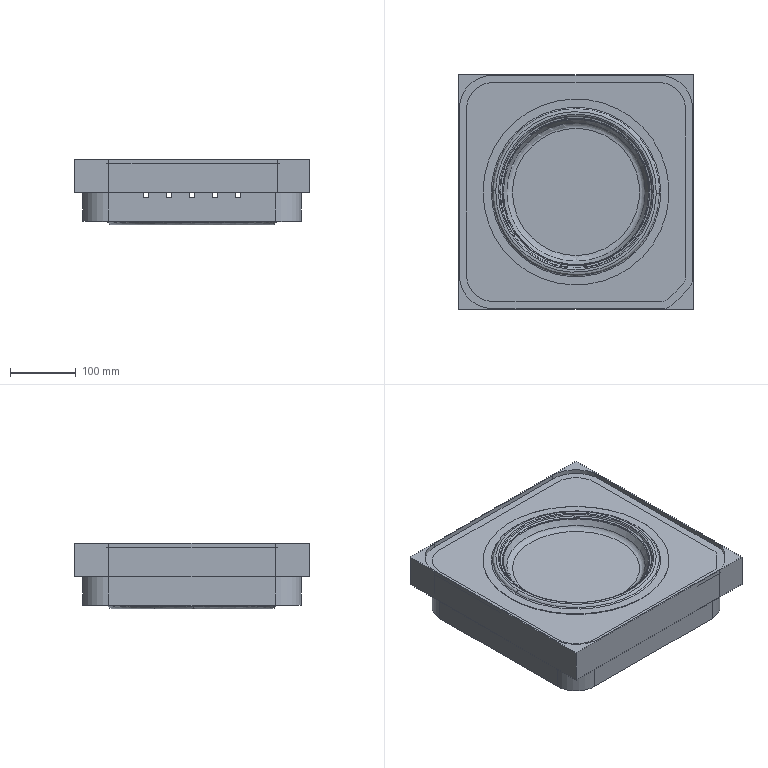NC program | NX | posted with a generic post | part box 356 x 356 x 99.5 mm
Lines 4524 to 5551 of 165566:
(2 , TOOL : D8)
N9046 M6
N9048 G53
N9050 G17 G0 G90 X-104.848 Y1.6 S7000 M3 M8
N9052 G43 Z200.5 H0
N9054 Z48.885
N9056 G94 G1 Z47.885 F4500.
N9058 X-110.089
N9060 G3 X-111.689 Y0. R1.6
N9062 G2 X0. Y111.689 R111.689
N9064 X-111.689 Y0. R-111.689
N9066 G3 X-110.089 Y-1.6 R1.6
N9068 G1 X-104.848
N9070 Z48.885
N9072 G0 Z53.5
N9074 X-104.658 Y1.6
N9076 Z48.556
N9078 G1 Z47.556
N9080 X-109.899
N9082 G3 X-111.499 Y0. R1.6
N9084 G2 X0. Y111.499 R111.499
N9086 X-111.499 Y0. R-111.499
N9088 G3 X-109.899 Y-1.6 R1.6
N9090 G1 X-104.658
N9092 Z48.556
N9094 G0 Z50.885
N9096 X-104.468 Y1.6
N9098 Z48.227
N9100 G1 Z47.227
N9102 X-109.709
N9104 G3 X-111.309 Y0. R1.6
N9106 G2 X0. Y111.309 R111.309
N9108 X-111.309 Y0. R-111.309
N9110 G3 X-109.709 Y-1.6 R1.6
N9112 G1 X-104.468
N9114 Z48.227
N9116 G0 Z50.556
N9118 X-104.278 Y1.6
N9120 Z47.898
N9122 G1 Z46.898
N9124 X-109.519
N9126 G3 X-111.119 Y0. R1.6
N9128 G2 X0. Y111.119 R111.119
N9130 X-111.119 Y0. R-111.119
N9132 G3 X-109.519 Y-1.6 R1.6
N9134 G1 X-104.278
N9136 Z47.898
N9138 G0 Z50.227
N9140 X-104.088 Y1.6
N9142 Z47.569
N9144 G1 Z46.569
N9146 X-109.329
N9148 G3 X-110.929 Y0. R1.6
N9150 G2 X0. Y110.929 R110.929
N9152 X-110.929 Y0. R-110.929
N9154 G3 X-109.329 Y-1.6 R1.6
N9156 G1 X-104.088
N9158 Z47.569
N9160 G0 Z49.898
N9162 X-103.898 Y1.6
N9164 Z47.24
N9166 G1 Z46.24
N9168 X-109.139
N9170 G3 X-110.739 Y0. R1.6
N9172 G2 X0. Y110.739 R110.739
N9174 X-110.739 Y0. R-110.739
N9176 G3 X-109.139 Y-1.6 R1.6
N9178 G1 X-103.898
N9180 Z47.24
N9182 G0 Z49.569
N9184 X-103.709 Y1.6
N9186 Z46.912
N9188 G1 Z45.912
N9190 X-108.945
N9192 G3 X-110.545 Y0. R1.6
N9194 G2 X-0.001 Y110.544 R110.544
N9196 X-110.545 Y0. R-110.544
N9198 G3 X-108.945 Y-1.6 R1.6
N9200 G1 X-103.709
N9202 Z46.912
N9204 G0 Z49.24
N9206 X-102.188 Y1.603
N9208 Z45.678
N9210 G1 Z44.678
N9212 X-107.536
N9214 G3 X-109.136 Y0.003 R1.6
N9216 G2 X1.037 Y109.135 R109.137
N9218 X-55.168 Y-94.163 R-109.134
N9220 X-109.136 Y0.003 R109.137
N9222 G3 X-107.536 Y-1.597 R1.6
N9224 G1 X-102.188
N9226 Z45.678
N9228 G0 Z48.912
N9230 X-72.173 Y-71.373
N9232 Z45.43
N9234 G1 Z44.43
N9236 X-74.264 Y-73.563
N9238 G3 X-74.211 Y-75.825 R1.6
N9240 G1 X-74.196 Y-75.839
N9242 X-74.124 Y-75.908
N9244 G2 X-74.044 Y-78.71 R2.
N9246 G1 X-74.333 Y-78.471
N9248 G3 X-75.025 Y-77.815 R1.538
N9250 G1 X-75.201 Y-77.546
N9252 G2 X-75.894 Y-76.854 R1.441
N9254 X-76.588 Y-76.161 R1.385
N9256 X-77.065 Y-75.802 R1.351
N9258 X-74.299 Y-75.742 R2.
N9260 G1 X-74.211 Y-75.825
N9262 G3 X-71.949 Y-75.772 R1.6
N9264 G1 X-69.853 Y-73.577
N9266 Z45.43
N9268 G0 Z47.678
N9270 X-81.623 Y-60.305
N9272 Z45.43
N9274 G1 Z44.43
N9276 X-83.973 Y-62.37
N9278 G3 X-84.119 Y-64.628 R1.6
N9280 G2 X-83.74 Y-65.106 R6.
N9282 G1 X-83.736 Y-65.111
N9284 G2 X-84.133 Y-67.849 R2.
N9286 X-85.037 Y-66.468 R4.255
N9288 X-86.197 Y-65.083 R2.208
N9290 G1 X-87.205 Y-63.867
N9292 X-87.208 Y-63.839
N9294 G2 X-84.529 Y-64.167 R2.
N9296 G1 X-84.513 Y-64.186
N9298 X-84.147 Y-64.596
N9300 X-84.119 Y-64.628
N9302 G3 X-81.861 Y-64.774 R1.6
N9304 G1 X-79.552 Y-62.744
N9306 Z45.43
N9308 G0 Z47.678
N9310 X-86.432 Y-55.045
N9312 Z45.43
N9314 G1 Z44.43
N9316 X-89.726 Y-57.437
N9318 G3 X-90.08 Y-59.672 R1.6
N9320 X-89.644 Y-60.237 R12.243
N9322 G1 X-89.545 Y-60.542
N9324 X-88.803 Y-61.612
N9326 X-88.76 Y-61.622
N9328 G3 X-87.674 Y-63.006 R6.708
N9330 X-87.609 Y-63.24 R1.008
N9332 X-86.562 Y-63.67 R0.8
N9334 G1 X-80.716 Y-61.232
N9336 Z45.43
N9338 G0 Z47.678
N9340 X-101.427 Y-1.782
N9342 Z45.43
N9344 G1 Z44.43
N9346 X-104.501 Y-1.819
N9348 G3 X-106.081 Y-3.439 R1.6
N9350 G1 X-106.08 Y-3.463
N9352 X-106.079 Y-3.492
N9354 X-106.062 Y-3.809
N9356 G2 X-107.906 Y-5.913 R2.
N9358 X-108.01 Y-4.154 R7.554
N9360 X-107.821 Y-2.077 R3.211
N9362 G1 X-107.825 Y-1.149
N9364 G2 X-106.093 Y-3.068 R2.
N9366 G1 X-106.081 Y-3.439
N9368 G3 X-104.431 Y-4.987 R1.6
N9370 G1 X-101.328 Y-4.888
N9372 Z45.43
N9374 G0 Z47.678
N9376 X-93.646 Y39.774
N9378 Z45.43
N9380 G1 Z44.43
N9382 X-97.306 Y42.148
N9384 G3 X-99.519 Y41.676 R1.6
N9386 G2 X-99.917 Y41.235 R1.875
N9388 G1 X-100.618 Y39.465
N9390 G2 X-101.3 Y37.709 R2.193
N9392 G1 X-101.335 Y37.529
N9394 G3 X-100.07 Y35.653 R1.6
N9396 G1 X-95.614 Y34.786
N9398 Z45.43
N9400 G0 Z47.678
N9402 X-86.878 Y53.863
N9404 Z45.43
N9406 G1 Z44.43
N9408 X-90.305 Y56.034
N9410 G3 X-92.513 Y55.539 R1.6
N9412 G2 X-93.003 Y55.085 R1.302
N9414 X-93.694 Y53.898 R2.033
N9416 X-94.4 Y52.621 R1.816
N9418 G3 X-94.674 Y52.135 R91.572
N9420 X-94.056 Y49.958 R1.6
N9422 G1 X-90.413 Y47.925
N9424 Z45.43
N9426 G0 Z47.678
N9428 X-76.192 Y67.144
N9430 Z45.43
N9432 G1 Z44.43
N9434 X-78.599 Y69.004
N9436 G3 X-80.844 Y68.716 R1.6
N9438 G2 X-80.991 Y68.533 R6.
N9440 X-83.751 Y68.237 R2.
N9442 G1 X-83.453 Y68.545
N9444 G2 X-82.858 Y69.238 R1.082
N9446 X-81.743 Y70.622 R3.617
N9448 X-80.987 Y71.544 R41.003
N9450 X-80.704 Y68.905 R2.
N9452 X-80.844 Y68.716 R6.
N9454 G3 X-80.556 Y66.472 R1.6
N9456 G1 X-78.149 Y64.612
N9458 Z45.43
N9460 G0 Z47.678
N9462 X-75.686 Y68.627
N9464 Z45.43
N9466 G1 Z44.43
N9468 X-78.97 Y71.372
N9470 G3 X-79.077 Y73.632 R1.6
N9472 G1 X-79.087 Y73.641
N9474 G2 X-77.94 Y74.777 R41.003
N9476 X-77.273 Y75.469 R1.379
N9478 X-76.586 Y76.161 R1.377
N9480 X-75.894 Y76.854 R1.384
N9482 X-75.202 Y77.546 R1.411
N9484 X-74.038 Y78.698 R18.413
N9486 X-74.125 Y75.911 R2.
N9488 G1 X-74.204 Y75.835
N9490 X-74.298 Y75.746
N9492 G2 X-75.602 Y75.214 R2.
N9494 X-76.161 Y73.861 R2.
N9496 G1 X-76.29 Y73.726
N9498 G2 X-79.077 Y73.632 R2.
N9500 G3 X-76.817 Y73.74 R1.6
N9502 G1 X-73.96 Y69.454
N9504 Z45.43
N9506 G0 Z47.678
N9508 X72.302 Y71.298
N9510 Z45.43
N9512 G1 Z44.43
N9514 X74.217 Y73.967
N9516 G3 X73.85 Y76.2 R1.6
N9518 G2 X73.63 Y76.383 R2.
N9520 G1 X73.374 Y76.629
N9522 G2 X73.289 Y79.426 R2.
N9524 X74.488 Y78.239 R52.149
N9526 X75.201 Y77.546 R1.572
N9528 X75.894 Y76.854 R1.441
N9530 X76.588 Y76.161 R1.385
N9532 X77.065 Y75.802 R1.351
N9534 X74.298 Y75.743 R2.
N9536 G1 X74.196 Y75.839
N9538 X74.124 Y75.908
N9540 G2 X73.898 Y76.167 R2.
N9542 G1 X73.85 Y76.2
N9544 G3 X71.617 Y75.833 R1.6
N9546 G1 X69.849 Y73.368
N9548 Z45.43
N9550 G0 Z47.678
N9552 X87.184 Y-51.825
N9554 Z45.43
N9556 G1 Z44.43
N9558 X89.811 Y-53.377
N9560 G3 X92.002 Y-52.814 R1.6
N9562 G1 X92.026 Y-52.774
N9564 X92.164 Y-52.544
N9566 G2 X94.85 Y-51.828 R2.
N9568 X93.632 Y-54.005 R113.525
N9570 G3 X93.003 Y-55.085 R1.963
N9572 G1 X92.822 Y-55.39
N9574 X92.599 Y-55.733
N9576 G2 X91.85 Y-53.088 R2.
N9578 X92.002 Y-52.814 R6.
N9580 G3 X91.439 Y-50.622 R1.6
N9582 G1 X88.794 Y-49.059
N9584 Z45.43
N9586 G0 Z47.678
N9588 X75.283 Y-68.769
N9590 Z45.43
N9592 G1 Z44.43
N9594 X78.729 Y-71.73
N9596 G3 X80.986 Y-71.56 R1.6
N9598 X81.77 Y-70.622 R46.024
N9600 X82.858 Y-69.238 R3.911
N9602 X83.453 Y-68.545 R1.082
N9604 G1 X83.737 Y-68.251
N9606 G3 X83.698 Y-65.988 R1.6
N9608 G1 X80.851 Y-63.238
N9610 Z45.43
N9612 G0 Z47.678
N9614 X69.743 Y-73.494
N9616 Z45.43
N9618 G1 Z44.43
N9620 X71.949 Y-75.785
N9622 G3 X74.211 Y-75.828 R1.6
N9624 G1 X74.298 Y-75.746
N9626 G2 X75.602 Y-75.214 R2.
N9628 X76.16 Y-73.862 R2.
N9630 G1 X76.29 Y-73.727
N9632 G2 X79.085 Y-73.639 R2.
N9634 X77.94 Y-74.777 R46.024
N9636 X77.273 Y-75.469 R1.379
N9638 X76.586 Y-76.161 R1.377
N9640 X75.894 Y-76.854 R1.384
N9642 X75.202 Y-77.546 R1.411
N9644 X74.487 Y-78.239 R1.578
N9646 X73.317 Y-79.382 R76.235
N9648 X73.41 Y-76.602 R2.
N9650 G1 X73.602 Y-76.416
N9652 G2 X73.887 Y-76.188 R2.
N9654 X74.125 Y-75.911 R2.
N9656 G1 X74.204 Y-75.835
N9658 X74.211 Y-75.828
N9660 G3 X74.254 Y-73.565 R1.6
N9662 G1 X72.068 Y-71.296
N9664 Z45.43
N9666 G0 Z47.678
N9668 X68.021 Y-71.79
N9670 Z44.242
N9672 G1 Z43.242
N9674 X71.704 Y-75.554
N9676 G3 X73.967 Y-75.578 R1.6
N9678 G2 X-75.578 Y-73.967 R105.75
N9680 X73.967 Y-75.578 R-105.75
N9682 G3 X73.991 Y-73.316 R1.6
N9684 G1 X70.308 Y-69.552
N9686 Z44.242
N9688 G0 Z47.43
N9690 X67.883 Y-71.649
N9692 Z43.9
N9694 G1 Z42.9
N9696 X71.566 Y-75.413
N9698 G3 X73.829 Y-75.437 R1.6
N9700 G2 X-75.437 Y-73.829 R105.553
N9702 X73.829 Y-75.437 R-105.553
N9704 G3 X73.853 Y-73.175 R1.6
N9706 G1 X70.17 Y-69.411
N9708 Z43.9
N9710 G0 Z46.242
N9712 X67.745 Y-71.508
N9714 Z43.559
N9716 G1 Z42.559
N9718 X71.428 Y-75.272
N9720 G3 X73.691 Y-75.296 R1.6
N9722 G2 X-75.296 Y-73.691 R105.356
N9724 X73.691 Y-75.296 R-105.356
N9726 G3 X73.715 Y-73.034 R1.6
N9728 G1 X70.032 Y-69.27
N9730 Z43.559
N9732 G0 Z45.9
N9734 X67.607 Y-71.367
N9736 Z43.217
N9738 G1 Z42.217
N9740 X71.29 Y-75.131
N9742 G3 X73.553 Y-75.155 R1.6
N9744 G2 X-75.155 Y-73.553 R105.159
N9746 X73.553 Y-75.155 R-105.159
N9748 G3 X73.577 Y-72.893 R1.6
N9750 G1 X69.894 Y-69.129
N9752 Z43.217
N9754 G0 Z45.559
N9756 X67.469 Y-71.226
N9758 Z42.875
N9760 G1 Z41.875
N9762 X71.152 Y-74.99
N9764 G3 X73.415 Y-75.014 R1.6
N9766 G2 X-75.014 Y-73.415 R104.962
N9768 X73.415 Y-75.014 R-104.962
N9770 G3 X73.439 Y-72.752 R1.6
N9772 G1 X69.756 Y-68.988
N9774 Z42.875
N9776 G0 Z45.217
N9778 X67.331 Y-71.085
N9780 Z42.534
N9782 G1 Z41.534
N9784 X71.014 Y-74.849
N9786 G3 X73.277 Y-74.873 R1.6
N9788 G2 X-74.873 Y-73.277 R104.764
N9790 X73.277 Y-74.873 R-104.764
N9792 G3 X73.301 Y-72.611 R1.6
N9794 G1 X69.618 Y-68.847
N9796 Z42.534
N9798 G0 Z44.875
N9800 X67.193 Y-70.944
N9802 Z42.192
N9804 G1 Z41.192
N9806 X70.877 Y-74.708
N9808 G3 X73.139 Y-74.733 R1.6
N9810 G2 X-74.733 Y-73.139 R104.567
N9812 X73.139 Y-74.733 R-104.567
N9814 G3 X73.164 Y-72.47 R1.6
N9816 G1 X69.48 Y-68.706
N9818 Z42.192
N9820 G0 Z44.534
N9822 X67.055 Y-70.804
N9824 Z41.851
N9826 G1 Z40.851
N9828 X70.739 Y-74.567
N9830 G3 X73.001 Y-74.592 R1.6
N9832 G2 X-74.592 Y-73.001 R104.37
N9834 X73.001 Y-74.592 R-104.37
N9836 G3 X73.026 Y-72.329 R1.6
N9838 G1 X69.342 Y-68.565
N9840 Z41.851
N9842 G0 Z44.192
N9844 X66.917 Y-70.663
N9846 Z41.509
N9848 G1 Z40.509
N9850 X70.601 Y-74.426
N9852 G3 X72.863 Y-74.451 R1.6
N9854 G2 X-74.451 Y-72.863 R104.173
N9856 X72.863 Y-74.451 R-104.173
N9858 G3 X72.888 Y-72.188 R1.6
N9860 G1 X69.204 Y-68.424
N9862 Z41.509
N9864 G0 Z43.851
N9866 X66.779 Y-70.522
N9868 Z41.168
N9870 G1 Z40.168
N9872 X70.463 Y-74.285
N9874 G3 X72.725 Y-74.31 R1.6
N9876 G2 X-74.31 Y-72.725 R103.976
N9878 X72.725 Y-74.31 R-103.976
N9880 G3 X72.75 Y-72.047 R1.6
N9882 G1 X69.066 Y-68.283
N9884 Z41.168
N9886 G0 Z43.509
N9888 X66.641 Y-70.381
N9890 Z40.826
N9892 G1 Z39.826
N9894 X70.325 Y-74.144
N9896 G3 X72.587 Y-74.169 R1.6
N9898 G2 X-74.169 Y-72.587 R103.778
N9900 X72.587 Y-74.169 R-103.778
N9902 G3 X72.612 Y-71.906 R1.6
N9904 G1 X68.928 Y-68.142
N9906 Z40.826
N9908 G0 Z43.168
N9910 X66.503 Y-70.24
N9912 Z40.484
N9914 G1 Z39.484
N9916 X70.187 Y-74.003
N9918 G3 X72.449 Y-74.028 R1.6
N9920 G2 X-74.028 Y-72.449 R103.581
N9922 X72.449 Y-74.028 R-103.581
N9924 G3 X72.474 Y-71.765 R1.6
N9926 G1 X68.79 Y-68.001
N9928 Z40.484
N9930 G0 Z42.826
N9932 X66.365 Y-70.099
N9934 Z40.143
N9936 G1 Z39.143
N9938 X70.049 Y-73.862
N9940 G3 X72.312 Y-73.887 R1.6
N9942 G2 X-73.887 Y-72.312 R103.384
N9944 X72.312 Y-73.887 R-103.384
N9946 G3 X72.336 Y-71.624 R1.6
N9948 G1 X68.652 Y-67.86
N9950 Z40.143
N9952 G0 Z42.484
N9954 X66.227 Y-69.958
N9956 Z39.801
N9958 G1 Z38.801
N9960 X69.911 Y-73.722
N9962 G3 X72.174 Y-73.746 R1.6
N9964 G2 X-73.746 Y-72.174 R103.187
N9966 X72.174 Y-73.746 R-103.187
N9968 G3 X72.198 Y-71.483 R1.6
N9970 G1 X68.514 Y-67.72
N9972 Z39.801
N9974 G0 Z42.143
N9976 X66.089 Y-69.817
N9978 Z39.46
N9980 G1 Z38.46
N9982 X69.773 Y-73.581
N9984 G3 X72.036 Y-73.605 R1.6
N9986 G2 X-73.605 Y-72.036 R102.989
N9988 X72.036 Y-73.605 R-102.989
N9990 G3 X72.06 Y-71.342 R1.6
N9992 G1 X68.376 Y-67.579
N9994 Z39.46
N9996 G0 Z41.801
N9998 X65.952 Y-69.676
N10000 Z39.118
N10002 G1 Z38.118
N10004 X69.635 Y-73.44
N10006 G3 X71.898 Y-73.464 R1.6
N10008 G2 X-73.464 Y-71.898 R102.792
N10010 X71.898 Y-73.464 R-102.792
N10012 G3 X71.922 Y-71.201 R1.6
N10014 G1 X68.239 Y-67.438
N10016 Z39.118
N10018 G0 Z41.46
N10020 X65.814 Y-69.535
N10022 Z38.776
N10024 G1 Z37.776
N10026 X69.497 Y-73.299
N10028 G3 X71.76 Y-73.323 R1.6
N10030 G2 X-73.323 Y-71.76 R102.595
N10032 X71.76 Y-73.323 R-102.595
N10034 G3 X71.784 Y-71.06 R1.6
N10036 G1 X68.101 Y-67.297
N10038 Z38.776
N10040 G0 Z41.118
N10042 X65.676 Y-69.394
N10044 Z38.435
N10046 G1 Z37.435
N10048 X69.359 Y-73.158
N10050 G3 X71.622 Y-73.182 R1.6
N10052 G2 X-73.182 Y-71.622 R102.398
N10054 X71.622 Y-73.182 R-102.398
N10056 G3 X71.646 Y-70.92 R1.6
N10058 G1 X67.963 Y-67.156
N10060 Z38.435
N10062 G0 Z40.776
N10064 X65.538 Y-69.253
N10066 Z38.093
N10068 G1 Z37.093
N10070 X69.221 Y-73.017
N10072 G3 X71.484 Y-73.041 R1.6
N10074 G2 X-73.041 Y-71.484 R102.201
N10076 X71.484 Y-73.041 R-102.201
N10078 G3 X71.508 Y-70.779 R1.6
N10080 G1 X67.825 Y-67.015
N10082 Z38.093
N10084 G0 Z40.435
N10086 X65.4 Y-69.112
N10088 Z37.752
N10090 G1 Z36.752
N10092 X69.083 Y-72.876
N10094 G3 X71.346 Y-72.9 R1.6
N10096 G2 X-72.9 Y-71.346 R102.003
N10098 X71.346 Y-72.9 R-102.003
N10100 G3 X71.37 Y-70.638 R1.6
N10102 G1 X67.687 Y-66.874
N10104 Z37.752
N10106 G0 Z40.093
N10108 X65.262 Y-68.971
N10110 Z37.41
N10112 G1 Z36.41
N10114 X68.945 Y-72.735
N10116 G3 X71.208 Y-72.759 R1.6
N10118 G2 X-72.759 Y-71.208 R101.806
N10120 X71.208 Y-72.759 R-101.806
N10122 G3 X71.232 Y-70.497 R1.6
N10124 G1 X67.549 Y-66.733
N10126 Z37.41
N10128 G0 Z39.752
N10130 X65.124 Y-68.83
N10132 Z37.069
N10134 G1 Z36.069
N10136 X68.807 Y-72.594
N10138 G3 X71.07 Y-72.618 R1.6
N10140 G2 X-72.618 Y-71.07 R101.609
N10142 X71.07 Y-72.618 R-101.609
N10144 G3 X71.094 Y-70.356 R1.6
N10146 G1 X67.411 Y-66.592
N10148 Z37.069
N10150 G0 Z39.41
N10152 X64.986 Y-68.689
N10154 Z36.727
N10156 G1 Z35.727
N10158 X68.67 Y-72.453
N10160 G3 X70.932 Y-72.477 R1.6
N10162 G2 X-72.477 Y-70.932 R101.412
N10164 X70.932 Y-72.477 R-101.412
N10166 G3 X70.957 Y-70.215 R1.6
N10168 G1 X67.273 Y-66.451
N10170 Z36.727
N10172 G0 Z39.069
N10174 X64.848 Y-68.548
N10176 Z36.385
N10178 G1 Z35.385
N10180 X68.532 Y-72.312
N10182 G3 X70.794 Y-72.336 R1.6
N10184 G2 X-72.336 Y-70.794 R101.215
N10186 X70.794 Y-72.336 R-101.215
N10188 G3 X70.819 Y-70.074 R1.6
N10190 G1 X67.135 Y-66.31
N10192 Z36.385
N10194 G0 Z38.727
N10196 X64.71 Y-68.407
N10198 Z36.044
N10200 G1 Z35.044
N10202 X68.394 Y-72.171
N10204 G3 X70.656 Y-72.196 R1.6
N10206 G2 X-72.196 Y-70.656 R101.017
N10208 X70.656 Y-72.196 R-101.017
N10210 G3 X70.681 Y-69.933 R1.6
N10212 G1 X66.997 Y-66.169
N10214 Z36.044
N10216 G0 Z38.385
N10218 X64.572 Y-68.266
N10220 Z35.702
N10222 G1 Z34.702
N10224 X68.255 Y-72.029
N10226 G3 X70.518 Y-72.054 R1.6
N10228 G2 X-72.054 Y-70.518 R100.819
N10230 X70.518 Y-72.054 R-100.819
N10232 G3 X70.542 Y-69.791 R1.6
N10234 G1 X66.859 Y-66.028
N10236 Z35.702
N10238 G0 Z38.044
N10240 X64.432 Y-68.123
N10242 Z35.361
N10244 G1 Z34.361
N10246 X68.106 Y-71.877
N10248 G3 X70.368 Y-71.901 R1.6
N10250 G2 X-71.901 Y-70.368 R100.606
N10252 X70.368 Y-71.901 R-100.606
N10254 G3 X70.393 Y-69.639 R1.6
N10256 G1 X66.719 Y-65.885
N10258 Z35.361
N10260 G0 Z37.702
N10262 X64.279 Y-67.967
N10264 Z35.019
N10266 G1 Z34.019
N10268 X67.942 Y-71.71
N10270 G3 X70.205 Y-71.734 R1.6
N10272 G2 X-71.734 Y-70.205 R100.372
N10274 X70.205 Y-71.734 R-100.372
N10276 G3 X70.229 Y-69.472 R1.6
N10278 G1 X66.566 Y-65.729
N10280 Z35.019
N10282 G0 Z37.361
N10284 X64.111 Y-67.795
N10286 Z34.677
N10288 G1 Z33.677
N10290 X67.764 Y-71.527
N10292 G3 X70.026 Y-71.552 R1.6
N10294 G2 X-71.552 Y-70.026 R100.116
N10296 X70.026 Y-71.552 R-100.116
N10298 G3 X70.051 Y-69.289 R1.6
N10300 G1 X66.398 Y-65.557
N10302 Z34.677
N10304 G0 Z37.019
N10306 X88.103 Y-1.6
N10308 Z31.262
N10310 G1 Z30.262
N10312 X93.366
N10314 G3 X94.966 Y0. R1.6
N10316 G2 X0. Y-94.966 R94.966
N10318 X94.966 Y0. R-94.966
N10320 G3 X93.366 Y1.6 R1.6
N10322 G1 X88.103
N10324 Z31.262
N10326 G0 Z52.2
N10328 X137.025 Y1.598
N10330 Z47.569
N10332 G1 Z46.569
N10334 X131.798
N10336 G3 X130.198 Y-0.002 R1.6
N10338 G2 X-121.922 Y45.697 R-130.202
N10340 X72.7 Y108.011 R130.201
N10342 X130.198 Y-0.002 R130.202
N10344 G3 X131.798 Y-1.602 R1.6
N10346 G1 X137.026
N10348 Z47.569
N10350 G0 Z49.898
N10352 X137.211 Y1.598
N10354 Z47.24
N10356 G1 Z46.24
N10358 X131.995
N10360 G3 X130.395 Y-0.002 R1.6
N10362 G2 X-0.002 Y-130.395 R130.395
N10364 X130.395 Y-0.002 R-130.395
N10366 G3 X131.995 Y-1.602 R1.6
N10368 G1 X137.21
N10370 Z47.24
N10372 G0 Z49.569
N10374 X137.4 Y1.599
N10376 Z46.912
N10378 G1 Z45.912
N10380 X132.192 Y1.598
N10382 G3 X130.592 Y-0.002 R1.6
N10384 G2 X125.125 Y-37.388 R130.398
N10386 X80.069 Y-103.164 R130.701
N10388 X75.025 Y106.889 R-130.59
N10390 G1 X75.365 Y106.626
N10392 X75.716 Y106.403
N10394 G2 X95.769 Y88.773 R130.593
N10396 X129.34 Y18.002 R130.422
N10398 X130.592 Y-0.002 R130.398
N10400 G3 X132.193 Y-1.602 R1.6
N10402 G1 X137.394 Y-1.601
N10404 Z46.912
N10406 G0 Z49.24
N10408 X152.025 Y1.6
N10410 Z45.678
N10412 G1 Z44.678
N10414 X146.8
N10416 G3 X145.2 Y0. R1.6
N10418 G2 X0. Y-145.2 R145.2
N10420 X145.2 Y0. R-145.2
N10422 G3 X146.8 Y-1.6 R1.6
N10424 G1 X152.025
N10426 Z45.678
N10428 G0 Z47.925
N10430 X152.116 Y1.6
N10432 Z45.43
N10434 G1 Z44.43
N10436 X146.8
N10438 G3 X145.2 Y0. R1.6
N10440 G2 X0. Y-145.2 R145.2
N10442 X145.2 Y0. R-145.2
N10444 G3 X146.8 Y-1.6 R1.6
N10446 G1 X152.116
N10448 Z45.43
N10450 G0 Z47.678
N10452 X152.148 Y1.6
N10454 Z45.178
N10456 G1 Z44.178
N10458 X146.8
N10460 G3 X145.2 Y0. R1.6
N10462 G2 X0. Y-145.2 R145.2
N10464 X145.2 Y0. R-145.2
N10466 G3 X146.8 Y-1.6 R1.6
N10468 G1 X152.148
N10470 Z45.178
N10472 G0 Z47.43
N10474 X152.732 Y1.6
N10476 Z44.925
N10478 G1 Z43.925
N10480 X146.8
N10482 G3 X145.2 Y0. R1.6
N10484 G2 X0. Y-145.2 R145.2
N10486 X145.2 Y0. R-145.2
N10488 G3 X146.8 Y-1.6 R1.6
N10490 G1 X152.732
N10492 Z44.925
N10494 G0 Z47.925
N10496 X165.815 Y-3.493
N10498 Z45.678
N10500 G1 Z44.678
N10502 X171.2
N10504 G3 X172.8 Y-1.893 R1.6
N10506 G1 Y-129.787
N10508 G2 X166.415 Y-145.202 R21.8
N10510 G1 X145.202 Y-166.415
N10512 G2 X129.787 Y-172.8 R21.8
N10514 G1 X-126.
N10516 G2 X-172.8 Y-126. R46.8
N10518 G1 Y126.
N10520 G2 X-126. Y172.8 R46.8
N10522 G1 X126.
N10524 G2 X172.8 Y126. R46.8
N10526 G1 Y-1.893
N10528 G3 X171.2 Y-0.293 R1.6
N10530 G1 X165.815
N10532 Z45.678
N10534 G0 Z47.925
N10536 X165.843 Y-3.493
N10538 Z45.43
N10540 G1 Z44.43
N10542 X171.2
N10544 G3 X172.8 Y-1.893 R1.6
N10546 G1 Y-129.787
N10548 G2 X166.415 Y-145.202 R21.8
N10550 G1 X145.202 Y-166.415
N10552 G2 X129.787 Y-172.8 R21.8
N10554 G1 X-126.
N10556 G2 X-172.8 Y-126. R46.8
N10558 G1 Y126.
N10560 G2 X-126. Y172.8 R46.8
N10562 G1 X126.
N10564 G2 X172.8 Y126. R46.8
N10566 G1 Y-1.893
N10568 G3 X171.2 Y-0.293 R1.6
N10570 G1 X165.843
N10572 Z45.43
N10574 G0 Z47.678
N10576 Y-3.493
N10578 Z45.178
N10580 G1 Z44.178
N10582 X171.2
N10584 G3 X172.8 Y-1.893 R1.6
N10586 G1 Y-129.787
N10588 G2 X166.415 Y-145.202 R21.8
N10590 G1 X145.202 Y-166.415
N10592 G2 X129.787 Y-172.8 R21.8
N10594 G1 X-126.
N10596 G2 X-172.8 Y-126. R46.8
N10598 G1 Y126.
N10600 G2 X-126. Y172.8 R46.8
N10602 G1 X126.
N10604 G2 X172.8 Y126. R46.8
N10606 G1 Y-1.893
N10608 G3 X171.2 Y-0.293 R1.6
N10610 G1 X165.843
N10612 Z45.178
N10614 G0 Z47.43
N10616 X165.26 Y-3.493
N10618 Z44.925
N10620 G1 Z43.925
N10622 X171.2
N10624 G3 X172.8 Y-1.893 R1.6
N10626 G1 Y-129.787
N10628 G2 X166.415 Y-145.202 R21.8
N10630 G1 X145.202 Y-166.415
N10632 G2 X129.787 Y-172.8 R21.8
N10634 G1 X-126.
N10636 G2 X-172.8 Y-126. R46.8
N10638 G1 Y126.
N10640 G2 X-126. Y172.8 R46.8
N10642 G1 X126.
N10644 G2 X172.8 Y126. R46.8
N10646 G1 Y-1.893
N10648 G3 X171.2 Y-0.293 R1.6
N10650 G1 X165.26
N10652 Z44.925
N10654 G0 Z200.5
N10656 M9
N10658 M5
(03 , TOOL : D12)
N10660 M6
N10662 G53
N10664 G17 G0 G90 X-159.461 Y-156.125 S7000 M3 M8
N10666 G43 Z200.5 H0
N10668 Z45.725
N10670 G94 G1 X-162.236 Y-152.733 Z45.495 F4000.
N10672 X-164.72 Y-148.988 Z45.26
N10674 X-166.819 Y-145.013 Z45.024
N10676 X-168.511 Y-140.85 Z44.789
N10678 X-169.78 Y-136.538 Z44.553
N10680 X-170.612 Y-132.121 Z44.318
N10682 X-171. Y-127.643 Z44.082
N10684 Y-120.83 Z43.725
N10686 Y126.
N10688 G2 X-126. Y171. R45.
N10690 G1 X126.
N10692 G2 X171. Y126. R45.
N10694 G1 Y-129.787
N10696 G2 X165.142 Y-143.929 R20.
N10698 G1 X143.929 Y-165.142
N10700 G2 X129.787 Y-171. R20.
N10702 G1 X-126.
N10704 G2 X-171. Y-126. R45.
N10706 G1 Y-120.83
N10708 X-162.6
N10710 Y126.
N10712 G2 X-126. Y162.6 R36.6
N10714 G1 X126.
N10716 G2 X162.6 Y126. R36.6
N10718 G1 Y-129.787
N10720 G2 X159.202 Y-137.989 R11.6
N10722 G1 X137.989 Y-159.202
N10724 G2 X129.787 Y-162.6 R11.6
N10726 G1 X-126.
N10728 G2 X-162.6 Y-126. R36.6
N10730 G1 Y-120.83
N10732 X-154.2
N10734 Y126.
N10736 G2 X-126. Y154.2 R28.2
N10738 G1 X-29.122
N10740 Y145.8
N10742 G3 X-145.8 Y29.122 R148.68
N10744 G1 X-148.2 Y23.623
N10746 Y11.937
N10748 G2 X-146.856 Y23.216 R148.68
N10750 X-148.2 Y23.623 R6.
N10752 G1 X-145.8 Y29.122
N10754 Y126.
N10756 G2 X-126. Y145.8 R19.8
N10758 G1 X-29.122
N10760 X-23.216 Y146.856
N10762 G2 X-11.937 Y148.2 R148.68
N10764 G1 X-23.623
N10766 G2 X-23.216 Y146.856 R6.
N10768 G1 X-29.122 Y145.8
N10770 X-76.127 Y137.4
N10772 G3 X-137.4 Y76.127 R157.08
N10774 G1 X-139.166 Y68.962
N10776 X-137.4 Y76.127
N10778 Y126.
N10780 G2 X-126. Y137.4 R11.4
N10782 G1 X-76.127
N10784 X-103.647 Y129.
N10786 G3 X-129. Y103.647 R165.48
N10788 G1 X-131.095 Y97.514
N10790 X-129. Y103.647
N10792 Y126.
N10794 G2 X-126. Y129. R3.
N10796 G1 X-123.6
N10798 Y123.6
N10800 X-117.996
N10802 G3 X-123.6 Y117.996 R170.88
N10804 G1 Y123.6
N10806 Y129.
N10808 X-103.647
N10810 X-76.127 Y137.4
N10812 X-29.122 Y145.8
N10814 Y154.2
N10816 X126.
N10818 G2 X154.2 Y126. R28.2
N10820 G1 Y29.122
N10822 X145.8
N10824 G3 X29.122 Y145.8 R148.68
N10826 G1 X23.623 Y148.2
N10828 X11.937
N10830 G2 X23.216 Y146.856 R148.68
N10832 X23.623 Y148.2 R6.
N10834 G1 X29.122 Y145.8
N10836 X126.
N10838 G2 X145.8 Y126. R19.8
N10840 G1 Y29.122
N10842 X146.856 Y23.216
N10844 G2 X148.2 Y11.937 R148.68
N10846 G1 Y23.623
N10848 G2 X146.856 Y23.216 R6.
N10850 G1 X145.8 Y29.122
N10852 X137.4 Y76.127
N10854 G3 X76.127 Y137.4 R157.08
N10856 G1 X68.962 Y139.166
N10858 X76.127 Y137.4
N10860 X126.
N10862 G2 X137.4 Y126. R11.4
N10864 G1 Y76.127
N10866 X129. Y103.647
N10868 G3 X103.647 Y129. R165.48
N10870 G1 X97.514 Y131.095
N10872 X103.647 Y129.
N10874 X126.
N10876 G2 X129. Y126. R3.
N10878 G1 Y123.6
N10880 X123.6
N10882 Y117.996
N10884 G3 X117.996 Y123.6 R170.88
N10886 G1 X123.6
N10888 X129.
N10890 Y103.647
N10892 X137.4 Y76.127
N10894 X145.8 Y29.122
N10896 X154.2
N10898 Y-129.787
N10900 G2 X153.263 Y-132.05 R3.2
N10902 G1 X132.05 Y-153.263
N10904 G2 X129.787 Y-154.2 R3.2
N10906 G1 X29.122
N10908 Y-145.8
N10910 G3 X145.8 Y-29.122 R148.68
N10912 G1 X148.2 Y-23.623
N10914 Y-11.937
N10916 G2 X146.856 Y-23.216 R148.68
N10918 X148.2 Y-23.623 R6.
N10920 G1 X145.8 Y-29.122
N10922 Y-127.633
N10924 X127.633 Y-145.8
N10926 X29.122
N10928 X23.216 Y-146.856
N10930 G2 X11.937 Y-148.2 R148.68
N10932 G1 X23.623
N10934 G2 X23.216 Y-146.856 R6.
N10936 G1 X29.122 Y-145.8
N10938 X76.127 Y-137.4
N10940 G3 X137.4 Y-76.127 R157.08
N10942 G1 X139.166 Y-68.962
N10944 X137.4 Y-76.127
N10946 Y-124.153
N10948 X124.153 Y-137.4
N10950 X76.127
N10952 X103.647 Y-129.
N10954 G3 X129. Y-103.647 R165.48
N10956 G1 X131.095 Y-97.514
N10958 X129. Y-103.647
N10960 Y-120.674
N10962 X120.674 Y-129.
N10964 X103.647
N10966 X117.996 Y-123.6
N10968 G3 X123.6 Y-117.996 R170.88
N10970 G1 Y-118.437
N10972 X118.437 Y-123.6
N10974 X117.996
N10976 X103.647 Y-129.
N10978 X76.127 Y-137.4
N10980 X29.122 Y-145.8
N10982 Y-154.2
N10984 X-126.
N10986 G2 X-154.2 Y-126. R28.2
N10988 G1 Y-120.83
N10990 X-145.8
N10992 Y-29.122
N10994 X-146.856 Y-23.216
N10996 G2 X-148.2 Y-11.937 R148.68
N10998 G1 Y-23.623
N11000 G2 X-146.856 Y-23.216 R6.
N11002 G1 X-145.8 Y-29.122
N11004 G3 X-29.122 Y-145.8 R148.68
N11006 G1 X-23.623 Y-148.2
N11008 X-11.937
N11010 G2 X-23.216 Y-146.856 R148.68
N11012 X-23.623 Y-148.2 R6.
N11014 G1 X-29.122 Y-145.8
N11016 X-28.793 Y-144.153
N11018 G2 X-144.153 Y28.793 R147.
N11020 X-28.793 Y-144.153 R-147.
N11022 G1 X-29.122 Y-145.8
N11024 X-126.
N11026 G2 X-145.8 Y-126. R19.8
N11028 G1 Y-120.83
N11030 X-137.4
N11032 Y-76.127
N11034 X-139.166 Y-68.962
N11036 X-137.4 Y-76.127
N11038 G3 X-76.127 Y-137.4 R157.08
N11040 G1 X-68.962 Y-139.166
N11042 X-76.127 Y-137.4
N11044 X-126.
N11046 G2 X-137.4 Y-126. R11.4
N11048 G1 Y-120.83
N11050 X-129.
N11052 Y-103.647
N11054 X-131.095 Y-97.514
N11056 X-129. Y-103.647
N11058 G3 X-103.647 Y-129. R165.48
N11060 G1 X-97.514 Y-131.095
N11062 X-103.647 Y-129.
N11064 X-126.
N11066 G2 X-129. Y-126. R3.
N11068 G1 Y-120.83
N11070 X-123.6
N11072 Y-117.996
N11074 G3 X-117.996 Y-123.6 R170.88
N11076 G1 X-123.6
N11078 Y-120.83
N11080 G3 X-126. Y-118.43 R2.4
N11082 G1 Z44.725
N11084 G0 Z200.5
N11086 M9
N11088 M5